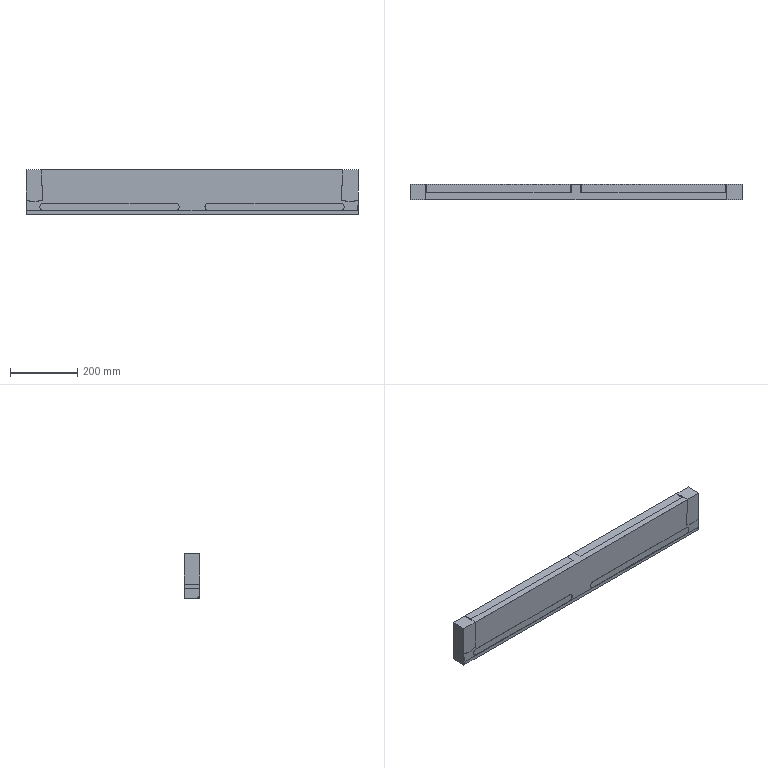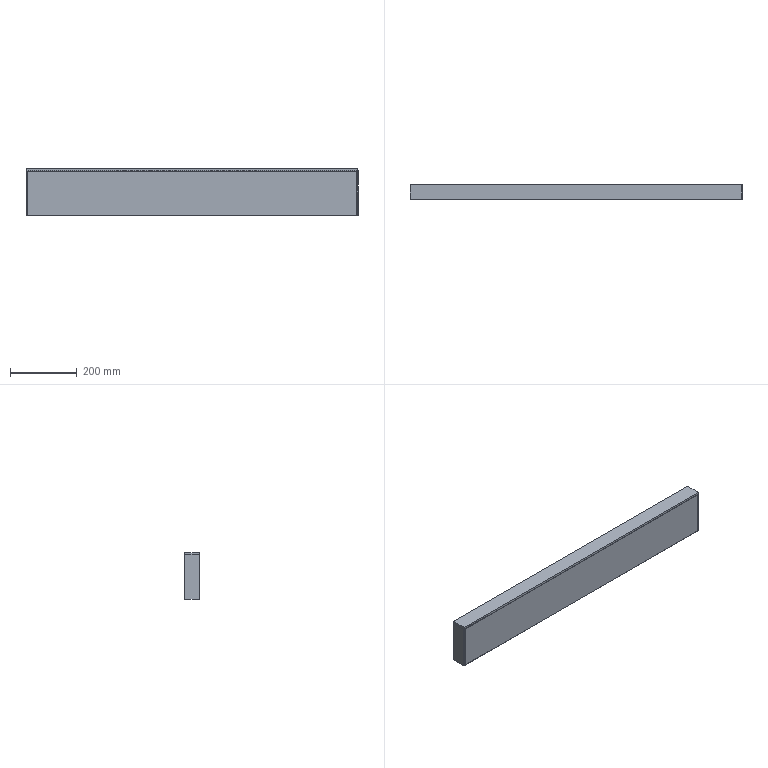CAM job | NX | 3+2 milling | part box 987 x 45 x 132.5 mm | stock box 997 x 45 x 140 mm
Tools:
number,name,description,diameter,corner_radius,flute_length,length,flutes
7,D10A45,Milling Tool-5 Parameters,10.0,0.0,5.0,5.0,2
1,D63,Milling Tool-5 Parameters,63.0,0.0,50.0,75.0,2
21,D12JING,Milling Tool-5 Parameters,12.0,0.0,50.0,75.0,2
16,D16,Milling Tool-5 Parameters,16.0,0.0,50.0,75.0,2
23,T50H10,Milling Tool-T Cutter,50.0,,10.0,25.0,4
20,D12,Milling Tool-5 Parameters,12.0,0.0,50.0,75.0,2
10,D10,Milling Tool-5 Parameters,10.0,0.0,50.0,75.0,2
11,D10JING,Milling Tool-5 Parameters,10.0,0.0,50.0,75.0,2
18,D12A45,Milling Tool-5 Parameters,12.0,0.0,6.0,6.0,2
9,D30INNERRCUTTER,User Defined Mill Tool,0.0,,10.0,54.0,2
Operations:
program,operation,operation_type,tool,method,geometry_group,spindle_rpm,surface_speed,feed_per_tooth,feed_cut,feed_plunge,cut_length_mm,path_length_mm,cut_time_min,machine_time_min
1,FLOOR_WALL,VolumeBased25DMillingOperation,D63,METHOD,A,6500.0,1286.0,0.0962,1250.0,100.0,1072.0,1126.0,0.8576,0.863
1,ZLEVEL_PROFILE_1_COPY_1_COPY_COPY_1,ZLevelMilling,D10A45,METHOD,A,7500.0,141.0,0.0667,1000.0,100.0,2019.507,2192.147,2.019,2.037
2,ZLEVEL_PROFILE_COPY_2,ZLevelMilling,D63,METHOD,MCS_MILL_B,6500.0,1021.0,0.1538,2000.0,100.0,4386.913,4446.913,2.193,2.2
2,ZLEVEL_PROFILE,ZLevelMilling,D63,METHOD,B,6500.0,1021.0,0.1538,2000.0,100.0,13750.242,15219.122,6.875,7.022
2,CUTTERCOMP9,ZLevelMilling,D16,METHOD,B,6500.0,326.0,0.0769,1000.0,100.0,430.933,1857.124,0.4309,0.5736
2,ZLEVEL_PROFILE_COPY,ZLevelMilling,D16,METHOD,B,6500.0,326.0,0.1538,2000.0,100.0,1122.521,3206.936,0.5613,0.7697
2,CUTTERCOMP9_COPY,ZLevelMilling,D16,METHOD,B,6500.0,326.0,0.0769,1000.0,100.0,287.332,2226.907,0.2873,0.4813
2,PLANAR_MILL_1,PlanarMilling,D10A45,METHOD,B,7500.0,141.0,0.0833,1250.0,100.0,1889.442,1945.442,1.512,1.517
2,ZLEVEL_PROFILE_1_COPY_1_COPY_COPY_1_COPY,ZLevelMilling,D12A45,METHOD,B,7000.0,219.0,0.0714,1000.0,100.0,286.851,2229.358,0.2869,0.4811
2,PLANAR_MILL,PlanarMilling,T50H10,METHOD,B,6000.0,942.0,0.0521,1250.0,100.0,7150.283,9016.79,3.801,3.987
3,ZLEVEL_PROFILE_COPY_1,ZLevelMilling,D12,METHOD,C,7500.0,235.0,0.2,3000.0,100.0,5276.359,6579.92,1.759,1.889
3,111,ZLevelMilling,D12JING,METHOD,C,6500.0,326.0,0.0769,1000.0,100.0,428.348,2375.513,0.4283,0.6231
3,FLOOR_WALL_1,VolumeBased25DMillingOperation,D10,METHOD,C,7500.0,0.0,0.0,3000.0,1000.0,20704.293,21778.976,6.91,7.018
3,FLOOR_WALL_2,VolumeBased25DMillingOperation,D10JING,METHOD,C,7000.0,219.0,0.0893,1250.0,100.0,4255.108,5632.096,3.404,3.542
3,ZLEVEL_PROFILE_1_COPY_1_COPY_COPY_1_COPY_1,ZLevelMilling,D10A45,METHOD,C,7500.0,141.0,0.0667,1000.0,100.0,1330.008,1391.008,1.33,1.336
3,ZLEVEL_PROFILE_1_COPY_1_COPY_COPY_1_COPY_1_COPY,ZLevelMilling,D10A45,METHOD,C,7500.0,141.0,0.0667,1000.0,100.0,848.343,1945.445,0.8483,0.9581
4,ZLEVEL_PROFILE_2,ZLevelMilling,D12,METHOD,D,7500.0,282.0,0.2,3000.0,1001.0,18181.771,19014.122,6.15,6.233
4,11,ZLevelMilling,D12,METHOD,D,6500.0,326.0,0.0769,1000.0,100.0,1637.604,2335.224,1.638,1.707
4,ZLEVEL_PROFILE_1_COPY_1_COPY_COPY_1_COPY_1_COPY_1,ZLevelMilling,D10A45,METHOD,D,7500.0,141.0,0.0667,1000.0,100.0,1699.044,2317.644,1.699,1.761
4,ZLEVEL_PROFILE_1_COPY_1_COPY_COPY_1_COPY_COPY,ZLevelMilling,D10A45,METHOD,D,7000.0,219.0,0.0714,1000.0,100.0,418.429,1526.053,0.4184,0.5292
4,PLANAR_PROFILE_COPY_COPY_COPY,PlanarMilling,D30INNERRCUTTER,METHOD,D,7500.0,0.0,0.0,1250.0,100.0,1002.909,1076.909,0.8023,0.8097
4,PLANAR_PROFILE_COPY_COPY_COPY_COPY,PlanarMilling,D30INNERRCUTTER,METHOD,D,7500.0,0.0,0.0,1250.0,100.0,1002.909,1076.909,0.8023,0.8097
4,PLANAR_PROFILE_COPY_COPY_COPY_COPY_COPY,PlanarMilling,D30INNERRCUTTER,METHOD,D,7500.0,0.0,0.0,1250.0,100.0,1002.909,1076.909,0.8023,0.8097
4,PLANAR_PROFILE_COPY_COPY_COPY_COPY_COPY_COPY,PlanarMilling,D30INNERRCUTTER,METHOD,D,7500.0,0.0,0.0,1250.0,100.0,1002.909,1076.909,0.8023,0.8097